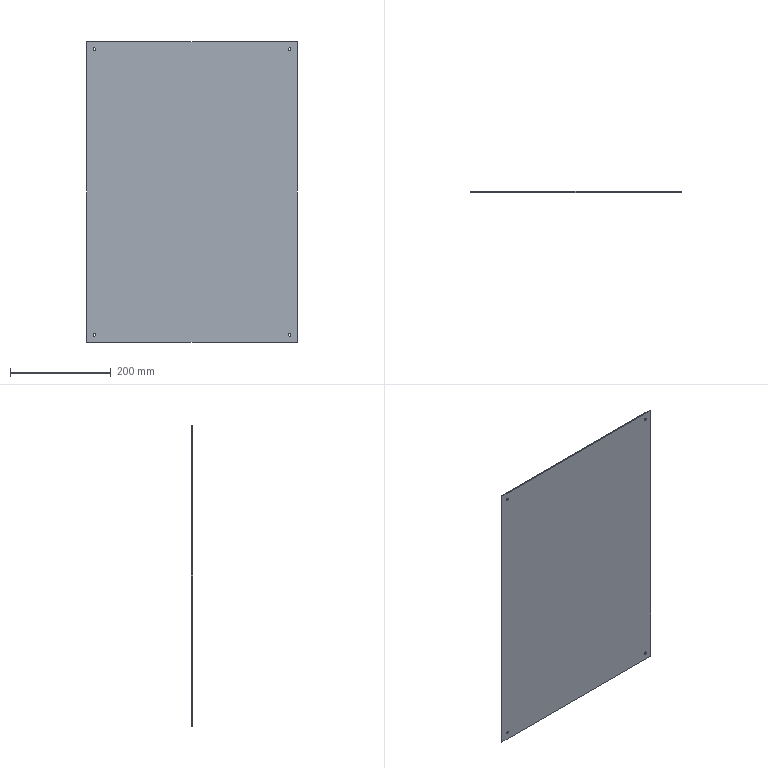Part | STEP file | PN_0007 (cover plate) | 1 solid | 14 faces | box 418 x 2 x 598 mm | volume 499771 mm3 | cylinder 8 | plane 6 | commonest cylinder face diameters 5 x8
STEP:
#1=CARTESIAN_POINT('',(0.,0.,0.));
#2=DIRECTION('',(0.,0.,1.));
#3=DIRECTION('',(1.,0.,0.));
#4=AXIS2_PLACEMENT_3D('',#1,#2,#3);
#5=CARTESIAN_POINT('',(-194.,-2.,286.5));
#6=VERTEX_POINT('',#5);
#7=CARTESIAN_POINT('',(-194.,0.,286.5));
#8=VERTEX_POINT('',#7);
#9=CARTESIAN_POINT('',(-194.,0.,286.5));
#10=DIRECTION('',(0.,1.,0.));
#11=VECTOR('',#10,1.);
#12=LINE('',#9,#11);
#13=CARTESIAN_POINT('',(-194.,0.,284.));
#14=DIRECTION('',(0.,1.,0.));
#15=DIRECTION('',(0.,0.,1.));
#16=AXIS2_PLACEMENT_3D('',#13,#14,#15);
#17=CYLINDRICAL_SURFACE('',#16,2.5);
#18=CARTESIAN_POINT('',(6.283,0.));
#19=DIRECTION('',(0.,1.));
#20=VECTOR('',#19,1.);
#21=LINE('',#18,#20);
#22=(GEOMETRIC_REPRESENTATION_CONTEXT(2)PARAMETRIC_REPRESENTATION_CONTEXT()REPRESENTATION_CONTEXT('',''));
#23=DEFINITIONAL_REPRESENTATION('',(#21),#22);
#24=PCURVE('',#17,#23);
#25=CARTESIAN_POINT('',(-194.,0.,284.));
#26=DIRECTION('',(0.,1.,0.));
#27=DIRECTION('',(0.,0.,1.));
#28=AXIS2_PLACEMENT_3D('',#25,#26,#27);
#29=CYLINDRICAL_SURFACE('',#28,2.5);
#30=CARTESIAN_POINT('',(0.,0.));
#31=DIRECTION('',(0.,1.));
#32=VECTOR('',#31,1.);
#33=LINE('',#30,#32);
#34=(GEOMETRIC_REPRESENTATION_CONTEXT(2)PARAMETRIC_REPRESENTATION_CONTEXT()REPRESENTATION_CONTEXT('',''));
#35=DEFINITIONAL_REPRESENTATION('',(#33),#34);
#36=PCURVE('',#29,#35);
#37=SURFACE_CURVE('',#12,(#24,#36),.PCURVE_S1.);
#38=EDGE_CURVE('',#6,#8,#37,.T.);
#39=ORIENTED_EDGE('',*,*,#38,.T.);
#40=CARTESIAN_POINT('',(-194.,0.,281.5));
#41=VERTEX_POINT('',#40);
#42=CARTESIAN_POINT('',(-194.,0.,284.));
#43=DIRECTION('',(0.,1.,0.));
#44=DIRECTION('',(0.,0.,1.));
#45=AXIS2_PLACEMENT_3D('',#42,#43,#44);
#46=CIRCLE('',#45,2.5);
#47=CARTESIAN_POINT('',(0.,0.));
#48=DIRECTION('',(1.,0.));
#49=VECTOR('',#48,1.);
#50=LINE('',#47,#49);
#51=(GEOMETRIC_REPRESENTATION_CONTEXT(2)PARAMETRIC_REPRESENTATION_CONTEXT()REPRESENTATION_CONTEXT('',''));
#52=DEFINITIONAL_REPRESENTATION('',(#50),#51);
#53=PCURVE('',#17,#52);
#54=CARTESIAN_POINT('',(0.,0.,0.));
#55=DIRECTION('',(0.,1.,0.));
#56=DIRECTION('',(0.,0.,1.));
#57=AXIS2_PLACEMENT_3D('',#54,#55,#56);
#58=PLANE('',#57);
#59=CARTESIAN_POINT('',(284.,-194.));
#60=DIRECTION('',(1.,0.));
#61=AXIS2_PLACEMENT_2D('',#59,#60);
#62=CIRCLE('',#61,2.5);
#63=(GEOMETRIC_REPRESENTATION_CONTEXT(2)PARAMETRIC_REPRESENTATION_CONTEXT()REPRESENTATION_CONTEXT('',''));
#64=DEFINITIONAL_REPRESENTATION('',(#62),#63);
#65=PCURVE('',#58,#64);
#66=SURFACE_CURVE('',#46,(#53,#65),.PCURVE_S1.);
#67=EDGE_CURVE('',#41,#8,#66,.T.);
#68=ORIENTED_EDGE('',*,*,#67,.F.);
#69=CARTESIAN_POINT('',(-194.,-2.,281.5));
#70=VERTEX_POINT('',#69);
#71=CARTESIAN_POINT('',(-194.,0.,281.5));
#72=DIRECTION('',(0.,1.,0.));
#73=VECTOR('',#72,1.);
#74=LINE('',#71,#73);
#75=CARTESIAN_POINT('',(3.142,0.));
#76=DIRECTION('',(0.,1.));
#77=VECTOR('',#76,1.);
#78=LINE('',#75,#77);
#79=(GEOMETRIC_REPRESENTATION_CONTEXT(2)PARAMETRIC_REPRESENTATION_CONTEXT()REPRESENTATION_CONTEXT('',''));
#80=DEFINITIONAL_REPRESENTATION('',(#78),#79);
#81=PCURVE('',#17,#80);
#82=CARTESIAN_POINT('',(3.142,0.));
#83=DIRECTION('',(0.,1.));
#84=VECTOR('',#83,1.);
#85=LINE('',#82,#84);
#86=(GEOMETRIC_REPRESENTATION_CONTEXT(2)PARAMETRIC_REPRESENTATION_CONTEXT()REPRESENTATION_CONTEXT('',''));
#87=DEFINITIONAL_REPRESENTATION('',(#85),#86);
#88=PCURVE('',#29,#87);
#89=SURFACE_CURVE('',#74,(#81,#88),.PCURVE_S1.);
#90=EDGE_CURVE('',#70,#41,#89,.T.);
#91=ORIENTED_EDGE('',*,*,#90,.F.);
#92=CARTESIAN_POINT('',(-194.,-2.,284.));
#93=DIRECTION('',(0.,1.,0.));
#94=DIRECTION('',(0.,0.,1.));
#95=AXIS2_PLACEMENT_3D('',#92,#93,#94);
#96=CIRCLE('',#95,2.5);
#97=CARTESIAN_POINT('',(0.,-2.));
#98=DIRECTION('',(1.,0.));
#99=VECTOR('',#98,1.);
#100=LINE('',#97,#99);
#101=(GEOMETRIC_REPRESENTATION_CONTEXT(2)PARAMETRIC_REPRESENTATION_CONTEXT()REPRESENTATION_CONTEXT('',''));
#102=DEFINITIONAL_REPRESENTATION('',(#100),#101);
#103=PCURVE('',#17,#102);
#104=CARTESIAN_POINT('',(0.,-2.,0.));
#105=DIRECTION('',(0.,1.,0.));
#106=DIRECTION('',(0.,0.,1.));
#107=AXIS2_PLACEMENT_3D('',#104,#105,#106);
#108=PLANE('',#107);
#109=CARTESIAN_POINT('',(284.,-194.));
#110=DIRECTION('',(1.,0.));
#111=AXIS2_PLACEMENT_2D('',#109,#110);
#112=CIRCLE('',#111,2.5);
#113=(GEOMETRIC_REPRESENTATION_CONTEXT(2)PARAMETRIC_REPRESENTATION_CONTEXT()REPRESENTATION_CONTEXT('',''));
#114=DEFINITIONAL_REPRESENTATION('',(#112),#113);
#115=PCURVE('',#108,#114);
#116=SURFACE_CURVE('',#96,(#103,#115),.PCURVE_S1.);
#117=EDGE_CURVE('',#70,#6,#116,.T.);
#118=ORIENTED_EDGE('',*,*,#117,.T.);
#119=EDGE_LOOP('',(#39,#68,#91,#118));
#120=FACE_BOUND('',#119,.F.);
#121=ADVANCED_FACE('',(#120),#17,.F.);
#122=CARTESIAN_POINT('',(194.,-2.,286.5));
#123=VERTEX_POINT('',#122);
#124=CARTESIAN_POINT('',(194.,0.,286.5));
#125=VERTEX_POINT('',#124);
#126=CARTESIAN_POINT('',(194.,0.,286.5));
#127=DIRECTION('',(0.,1.,0.));
#128=VECTOR('',#127,1.);
#129=LINE('',#126,#128);
#130=CARTESIAN_POINT('',(194.,0.,284.));
#131=DIRECTION('',(0.,1.,0.));
#132=DIRECTION('',(0.,0.,1.));
#133=AXIS2_PLACEMENT_3D('',#130,#131,#132);
#134=CYLINDRICAL_SURFACE('',#133,2.5);
#135=CARTESIAN_POINT('',(6.283,0.));
#136=DIRECTION('',(0.,1.));
#137=VECTOR('',#136,1.);
#138=LINE('',#135,#137);
#139=(GEOMETRIC_REPRESENTATION_CONTEXT(2)PARAMETRIC_REPRESENTATION_CONTEXT()REPRESENTATION_CONTEXT('',''));
#140=DEFINITIONAL_REPRESENTATION('',(#138),#139);
#141=PCURVE('',#134,#140);
#142=CARTESIAN_POINT('',(194.,0.,284.));
#143=DIRECTION('',(0.,1.,0.));
#144=DIRECTION('',(0.,0.,1.));
#145=AXIS2_PLACEMENT_3D('',#142,#143,#144);
#146=CYLINDRICAL_SURFACE('',#145,2.5);
#147=CARTESIAN_POINT('',(0.,0.));
#148=DIRECTION('',(0.,1.));
#149=VECTOR('',#148,1.);
#150=LINE('',#147,#149);
#151=(GEOMETRIC_REPRESENTATION_CONTEXT(2)PARAMETRIC_REPRESENTATION_CONTEXT()REPRESENTATION_CONTEXT('',''));
#152=DEFINITIONAL_REPRESENTATION('',(#150),#151);
#153=PCURVE('',#146,#152);
#154=SURFACE_CURVE('',#129,(#141,#153),.PCURVE_S1.);
#155=EDGE_CURVE('',#123,#125,#154,.T.);
#156=ORIENTED_EDGE('',*,*,#155,.T.);
#157=CARTESIAN_POINT('',(194.,0.,281.5));
#158=VERTEX_POINT('',#157);
#159=CARTESIAN_POINT('',(194.,0.,284.));
#160=DIRECTION('',(0.,1.,0.));
#161=DIRECTION('',(0.,0.,1.));
#162=AXIS2_PLACEMENT_3D('',#159,#160,#161);
#163=CIRCLE('',#162,2.5);
#164=CARTESIAN_POINT('',(0.,0.));
#165=DIRECTION('',(1.,0.));
#166=VECTOR('',#165,1.);
#167=LINE('',#164,#166);
#168=(GEOMETRIC_REPRESENTATION_CONTEXT(2)PARAMETRIC_REPRESENTATION_CONTEXT()REPRESENTATION_CONTEXT('',''));
#169=DEFINITIONAL_REPRESENTATION('',(#167),#168);
#170=PCURVE('',#134,#169);
#171=CARTESIAN_POINT('',(284.,194.));
#172=DIRECTION('',(1.,0.));
#173=AXIS2_PLACEMENT_2D('',#171,#172);
#174=CIRCLE('',#173,2.5);
#175=(GEOMETRIC_REPRESENTATION_CONTEXT(2)PARAMETRIC_REPRESENTATION_CONTEXT()REPRESENTATION_CONTEXT('',''));
#176=DEFINITIONAL_REPRESENTATION('',(#174),#175);
#177=PCURVE('',#58,#176);
#178=SURFACE_CURVE('',#163,(#170,#177),.PCURVE_S1.);
#179=EDGE_CURVE('',#158,#125,#178,.T.);
#180=ORIENTED_EDGE('',*,*,#179,.F.);
#181=CARTESIAN_POINT('',(194.,-2.,281.5));
#182=VERTEX_POINT('',#181);
#183=CARTESIAN_POINT('',(194.,0.,281.5));
#184=DIRECTION('',(0.,1.,0.));
#185=VECTOR('',#184,1.);
#186=LINE('',#183,#185);
#187=CARTESIAN_POINT('',(3.142,0.));
#188=DIRECTION('',(0.,1.));
#189=VECTOR('',#188,1.);
#190=LINE('',#187,#189);
#191=(GEOMETRIC_REPRESENTATION_CONTEXT(2)PARAMETRIC_REPRESENTATION_CONTEXT()REPRESENTATION_CONTEXT('',''));
#192=DEFINITIONAL_REPRESENTATION('',(#190),#191);
#193=PCURVE('',#134,#192);
#194=CARTESIAN_POINT('',(3.142,0.));
#195=DIRECTION('',(0.,1.));
#196=VECTOR('',#195,1.);
#197=LINE('',#194,#196);
#198=(GEOMETRIC_REPRESENTATION_CONTEXT(2)PARAMETRIC_REPRESENTATION_CONTEXT()REPRESENTATION_CONTEXT('',''));
#199=DEFINITIONAL_REPRESENTATION('',(#197),#198);
#200=PCURVE('',#146,#199);
#201=SURFACE_CURVE('',#186,(#193,#200),.PCURVE_S1.);
#202=EDGE_CURVE('',#182,#158,#201,.T.);
#203=ORIENTED_EDGE('',*,*,#202,.F.);
#204=CARTESIAN_POINT('',(194.,-2.,284.));
#205=DIRECTION('',(0.,1.,0.));
#206=DIRECTION('',(0.,0.,1.));
#207=AXIS2_PLACEMENT_3D('',#204,#205,#206);
#208=CIRCLE('',#207,2.5);
#209=CARTESIAN_POINT('',(0.,-2.));
#210=DIRECTION('',(1.,0.));
#211=VECTOR('',#210,1.);
#212=LINE('',#209,#211);
#213=(GEOMETRIC_REPRESENTATION_CONTEXT(2)PARAMETRIC_REPRESENTATION_CONTEXT()REPRESENTATION_CONTEXT('',''));
#214=DEFINITIONAL_REPRESENTATION('',(#212),#213);
#215=PCURVE('',#134,#214);
#216=CARTESIAN_POINT('',(284.,194.));
#217=DIRECTION('',(1.,0.));
#218=AXIS2_PLACEMENT_2D('',#216,#217);
#219=CIRCLE('',#218,2.5);
#220=(GEOMETRIC_REPRESENTATION_CONTEXT(2)PARAMETRIC_REPRESENTATION_CONTEXT()REPRESENTATION_CONTEXT('',''));
#221=DEFINITIONAL_REPRESENTATION('',(#219),#220);
#222=PCURVE('',#108,#221);
#223=SURFACE_CURVE('',#208,(#215,#222),.PCURVE_S1.);
#224=EDGE_CURVE('',#182,#123,#223,.T.);
#225=ORIENTED_EDGE('',*,*,#224,.T.);
#226=EDGE_LOOP('',(#156,#180,#203,#225));
#227=FACE_BOUND('',#226,.F.);
#228=ADVANCED_FACE('',(#227),#134,.F.);
#229=CARTESIAN_POINT('',(194.,-2.,-281.5));
#230=VERTEX_POINT('',#229);
#231=CARTESIAN_POINT('',(194.,0.,-281.5));
#232=VERTEX_POINT('',#231);
#233=CARTESIAN_POINT('',(194.,0.,-281.5));
#234=DIRECTION('',(0.,1.,0.));
#235=VECTOR('',#234,1.);
#236=LINE('',#233,#235);
#237=CARTESIAN_POINT('',(194.,0.,-284.));
#238=DIRECTION('',(0.,1.,0.));
#239=DIRECTION('',(0.,0.,1.));
#240=AXIS2_PLACEMENT_3D('',#237,#238,#239);
#241=CYLINDRICAL_SURFACE('',#240,2.5);
#242=CARTESIAN_POINT('',(6.283,0.));
#243=DIRECTION('',(0.,1.));
#244=VECTOR('',#243,1.);
#245=LINE('',#242,#244);
#246=(GEOMETRIC_REPRESENTATION_CONTEXT(2)PARAMETRIC_REPRESENTATION_CONTEXT()REPRESENTATION_CONTEXT('',''));
#247=DEFINITIONAL_REPRESENTATION('',(#245),#246);
#248=PCURVE('',#241,#247);
#249=CARTESIAN_POINT('',(194.,0.,-284.));
#250=DIRECTION('',(0.,1.,0.));
#251=DIRECTION('',(0.,0.,1.));
#252=AXIS2_PLACEMENT_3D('',#249,#250,#251);
#253=CYLINDRICAL_SURFACE('',#252,2.5);
#254=CARTESIAN_POINT('',(0.,0.));
#255=DIRECTION('',(0.,1.));
#256=VECTOR('',#255,1.);
#257=LINE('',#254,#256);
#258=(GEOMETRIC_REPRESENTATION_CONTEXT(2)PARAMETRIC_REPRESENTATION_CONTEXT()REPRESENTATION_CONTEXT('',''));
#259=DEFINITIONAL_REPRESENTATION('',(#257),#258);
#260=PCURVE('',#253,#259);
#261=SURFACE_CURVE('',#236,(#248,#260),.PCURVE_S1.);
#262=EDGE_CURVE('',#230,#232,#261,.T.);
#263=ORIENTED_EDGE('',*,*,#262,.T.);
#264=CARTESIAN_POINT('',(194.,0.,-286.5));
#265=VERTEX_POINT('',#264);
#266=CARTESIAN_POINT('',(194.,0.,-284.));
#267=DIRECTION('',(0.,1.,0.));
#268=DIRECTION('',(0.,0.,1.));
#269=AXIS2_PLACEMENT_3D('',#266,#267,#268);
#270=CIRCLE('',#269,2.5);
#271=CARTESIAN_POINT('',(0.,0.));
#272=DIRECTION('',(1.,0.));
#273=VECTOR('',#272,1.);
#274=LINE('',#271,#273);
#275=(GEOMETRIC_REPRESENTATION_CONTEXT(2)PARAMETRIC_REPRESENTATION_CONTEXT()REPRESENTATION_CONTEXT('',''));
#276=DEFINITIONAL_REPRESENTATION('',(#274),#275);
#277=PCURVE('',#241,#276);
#278=CARTESIAN_POINT('',(-284.,194.));
#279=DIRECTION('',(1.,0.));
#280=AXIS2_PLACEMENT_2D('',#278,#279);
#281=CIRCLE('',#280,2.5);
#282=(GEOMETRIC_REPRESENTATION_CONTEXT(2)PARAMETRIC_REPRESENTATION_CONTEXT()REPRESENTATION_CONTEXT('',''));
#283=DEFINITIONAL_REPRESENTATION('',(#281),#282);
#284=PCURVE('',#58,#283);
#285=SURFACE_CURVE('',#270,(#277,#284),.PCURVE_S1.);
#286=EDGE_CURVE('',#265,#232,#285,.T.);
#287=ORIENTED_EDGE('',*,*,#286,.F.);
#288=CARTESIAN_POINT('',(194.,-2.,-286.5));
#289=VERTEX_POINT('',#288);
#290=CARTESIAN_POINT('',(194.,0.,-286.5));
#291=DIRECTION('',(0.,1.,0.));
#292=VECTOR('',#291,1.);
#293=LINE('',#290,#292);
#294=CARTESIAN_POINT('',(3.142,0.));
#295=DIRECTION('',(0.,1.));
#296=VECTOR('',#295,1.);
#297=LINE('',#294,#296);
#298=(GEOMETRIC_REPRESENTATION_CONTEXT(2)PARAMETRIC_REPRESENTATION_CONTEXT()REPRESENTATION_CONTEXT('',''));
#299=DEFINITIONAL_REPRESENTATION('',(#297),#298);
#300=PCURVE('',#241,#299);
#301=CARTESIAN_POINT('',(3.142,0.));
#302=DIRECTION('',(0.,1.));
#303=VECTOR('',#302,1.);
#304=LINE('',#301,#303);
#305=(GEOMETRIC_REPRESENTATION_CONTEXT(2)PARAMETRIC_REPRESENTATION_CONTEXT()REPRESENTATION_CONTEXT('',''));
#306=DEFINITIONAL_REPRESENTATION('',(#304),#305);
#307=PCURVE('',#253,#306);
#308=SURFACE_CURVE('',#293,(#300,#307),.PCURVE_S1.);
#309=EDGE_CURVE('',#289,#265,#308,.T.);
#310=ORIENTED_EDGE('',*,*,#309,.F.);
#311=CARTESIAN_POINT('',(194.,-2.,-284.));
#312=DIRECTION('',(0.,1.,0.));
#313=DIRECTION('',(0.,0.,1.));
#314=AXIS2_PLACEMENT_3D('',#311,#312,#313);
#315=CIRCLE('',#314,2.5);
#316=CARTESIAN_POINT('',(0.,-2.));
#317=DIRECTION('',(1.,0.));
#318=VECTOR('',#317,1.);
#319=LINE('',#316,#318);
#320=(GEOMETRIC_REPRESENTATION_CONTEXT(2)PARAMETRIC_REPRESENTATION_CONTEXT()REPRESENTATION_CONTEXT('',''));
#321=DEFINITIONAL_REPRESENTATION('',(#319),#320);
#322=PCURVE('',#241,#321);
#323=CARTESIAN_POINT('',(-284.,194.));
#324=DIRECTION('',(1.,0.));
#325=AXIS2_PLACEMENT_2D('',#323,#324);
#326=CIRCLE('',#325,2.5);
#327=(GEOMETRIC_REPRESENTATION_CONTEXT(2)PARAMETRIC_REPRESENTATION_CONTEXT()REPRESENTATION_CONTEXT('',''));
#328=DEFINITIONAL_REPRESENTATION('',(#326),#327);
#329=PCURVE('',#108,#328);
#330=SURFACE_CURVE('',#315,(#322,#329),.PCURVE_S1.);
#331=EDGE_CURVE('',#289,#230,#330,.T.);
#332=ORIENTED_EDGE('',*,*,#331,.T.);
#333=EDGE_LOOP('',(#263,#287,#310,#332));
#334=FACE_BOUND('',#333,.F.);
#335=ADVANCED_FACE('',(#334),#241,.F.);
#336=CARTESIAN_POINT('',(-194.,-2.,-281.5));
#337=VERTEX_POINT('',#336);
#338=CARTESIAN_POINT('',(-194.,0.,-281.5));
#339=VERTEX_POINT('',#338);
#340=CARTESIAN_POINT('',(-194.,0.,-281.5));
#341=DIRECTION('',(0.,1.,0.));
#342=VECTOR('',#341,1.);
#343=LINE('',#340,#342);
#344=CARTESIAN_POINT('',(-194.,0.,-284.));
#345=DIRECTION('',(0.,1.,0.));
#346=DIRECTION('',(0.,0.,1.));
#347=AXIS2_PLACEMENT_3D('',#344,#345,#346);
#348=CYLINDRICAL_SURFACE('',#347,2.5);
#349=CARTESIAN_POINT('',(6.283,0.));
#350=DIRECTION('',(0.,1.));
#351=VECTOR('',#350,1.);
#352=LINE('',#349,#351);
#353=(GEOMETRIC_REPRESENTATION_CONTEXT(2)PARAMETRIC_REPRESENTATION_CONTEXT()REPRESENTATION_CONTEXT('',''));
#354=DEFINITIONAL_REPRESENTATION('',(#352),#353);
#355=PCURVE('',#348,#354);
#356=CARTESIAN_POINT('',(-194.,0.,-284.));
#357=DIRECTION('',(0.,1.,0.));
#358=DIRECTION('',(0.,0.,1.));
#359=AXIS2_PLACEMENT_3D('',#356,#357,#358);
#360=CYLINDRICAL_SURFACE('',#359,2.5);
#361=CARTESIAN_POINT('',(0.,0.));
#362=DIRECTION('',(0.,1.));
#363=VECTOR('',#362,1.);
#364=LINE('',#361,#363);
#365=(GEOMETRIC_REPRESENTATION_CONTEXT(2)PARAMETRIC_REPRESENTATION_CONTEXT()REPRESENTATION_CONTEXT('',''));
#366=DEFINITIONAL_REPRESENTATION('',(#364),#365);
#367=PCURVE('',#360,#366);
#368=SURFACE_CURVE('',#343,(#355,#367),.PCURVE_S1.);
#369=EDGE_CURVE('',#337,#339,#368,.T.);
#370=ORIENTED_EDGE('',*,*,#369,.T.);
#371=CARTESIAN_POINT('',(-194.,0.,-286.5));
#372=VERTEX_POINT('',#371);
#373=CARTESIAN_POINT('',(-194.,0.,-284.));
#374=DIRECTION('',(0.,1.,0.));
#375=DIRECTION('',(0.,0.,1.));
#376=AXIS2_PLACEMENT_3D('',#373,#374,#375);
#377=CIRCLE('',#376,2.5);
#378=CARTESIAN_POINT('',(0.,0.));
#379=DIRECTION('',(1.,0.));
#380=VECTOR('',#379,1.);
#381=LINE('',#378,#380);
#382=(GEOMETRIC_REPRESENTATION_CONTEXT(2)PARAMETRIC_REPRESENTATION_CONTEXT()REPRESENTATION_CONTEXT('',''));
#383=DEFINITIONAL_REPRESENTATION('',(#381),#382);
#384=PCURVE('',#348,#383);
#385=CARTESIAN_POINT('',(-284.,-194.));
#386=DIRECTION('',(1.,0.));
#387=AXIS2_PLACEMENT_2D('',#385,#386);
#388=CIRCLE('',#387,2.5);
#389=(GEOMETRIC_REPRESENTATION_CONTEXT(2)PARAMETRIC_REPRESENTATION_CONTEXT()REPRESENTATION_CONTEXT('',''));
#390=DEFINITIONAL_REPRESENTATION('',(#388),#389);
#391=PCURVE('',#58,#390);
#392=SURFACE_CURVE('',#377,(#384,#391),.PCURVE_S1.);
#393=EDGE_CURVE('',#372,#339,#392,.T.);
#394=ORIENTED_EDGE('',*,*,#393,.F.);
#395=CARTESIAN_POINT('',(-194.,-2.,-286.5));
#396=VERTEX_POINT('',#395);
#397=CARTESIAN_POINT('',(-194.,0.,-286.5));
#398=DIRECTION('',(0.,1.,0.));
#399=VECTOR('',#398,1.);
#400=LINE('',#397,#399);
#401=CARTESIAN_POINT('',(3.142,0.));
#402=DIRECTION('',(0.,1.));
#403=VECTOR('',#402,1.);
#404=LINE('',#401,#403);
#405=(GEOMETRIC_REPRESENTATION_CONTEXT(2)PARAMETRIC_REPRESENTATION_CONTEXT()REPRESENTATION_CONTEXT('',''));
#406=DEFINITIONAL_REPRESENTATION('',(#404),#405);
#407=PCURVE('',#348,#406);
#408=CARTESIAN_POINT('',(3.142,0.));
#409=DIRECTION('',(0.,1.));
#410=VECTOR('',#409,1.);
#411=LINE('',#408,#410);
#412=(GEOMETRIC_REPRESENTATION_CONTEXT(2)PARAMETRIC_REPRESENTATION_CONTEXT()REPRESENTATION_CONTEXT('',''));
#413=DEFINITIONAL_REPRESENTATION('',(#411),#412);
#414=PCURVE('',#360,#413);
#415=SURFACE_CURVE('',#400,(#407,#414),.PCURVE_S1.);
#416=EDGE_CURVE('',#396,#372,#415,.T.);
#417=ORIENTED_EDGE('',*,*,#416,.F.);
#418=CARTESIAN_POINT('',(-194.,-2.,-284.));
#419=DIRECTION('',(0.,1.,0.));
#420=DIRECTION('',(0.,0.,1.));
#421=AXIS2_PLACEMENT_3D('',#418,#419,#420);
#422=CIRCLE('',#421,2.5);
#423=CARTESIAN_POINT('',(0.,-2.));
#424=DIRECTION('',(1.,0.));
#425=VECTOR('',#424,1.);
#426=LINE('',#423,#425);
#427=(GEOMETRIC_REPRESENTATION_CONTEXT(2)PARAMETRIC_REPRESENTATION_CONTEXT()REPRESENTATION_CONTEXT('',''));
#428=DEFINITIONAL_REPRESENTATION('',(#426),#427);
#429=PCURVE('',#348,#428);
#430=CARTESIAN_POINT('',(-284.,-194.));
#431=DIRECTION('',(1.,0.));
#432=AXIS2_PLACEMENT_2D('',#430,#431);
#433=CIRCLE('',#432,2.5);
#434=(GEOMETRIC_REPRESENTATION_CONTEXT(2)PARAMETRIC_REPRESENTATION_CONTEXT()REPRESENTATION_CONTEXT('',''));
#435=DEFINITIONAL_REPRESENTATION('',(#433),#434);
#436=PCURVE('',#108,#435);
#437=SURFACE_CURVE('',#422,(#429,#436),.PCURVE_S1.);
#438=EDGE_CURVE('',#396,#337,#437,.T.);
#439=ORIENTED_EDGE('',*,*,#438,.T.);
#440=EDGE_LOOP('',(#370,#394,#417,#439));
#441=FACE_BOUND('',#440,.F.);
#442=ADVANCED_FACE('',(#441),#348,.F.);
#443=CARTESIAN_POINT('',(-209.,0.,299.));
#444=VERTEX_POINT('',#443);
#445=CARTESIAN_POINT('',(209.,0.,299.));
#446=VERTEX_POINT('',#445);
#447=CARTESIAN_POINT('',(209.,0.,299.));
#448=DIRECTION('',(1.,0.,0.));
#449=VECTOR('',#448,1.);
#450=LINE('',#447,#449);
#451=CARTESIAN_POINT('',(209.,-2.,299.));
#452=DIRECTION('',(0.,0.,1.));
#453=DIRECTION('',(1.,0.,0.));
#454=AXIS2_PLACEMENT_3D('',#451,#452,#453);
#455=PLANE('',#454);
#456=CARTESIAN_POINT('',(0.,2.));
#457=DIRECTION('',(1.,0.));
#458=VECTOR('',#457,1.);
#459=LINE('',#456,#458);
#460=(GEOMETRIC_REPRESENTATION_CONTEXT(2)PARAMETRIC_REPRESENTATION_CONTEXT()REPRESENTATION_CONTEXT('',''));
#461=DEFINITIONAL_REPRESENTATION('',(#459),#460);
#462=PCURVE('',#455,#461);
#463=CARTESIAN_POINT('',(299.,209.));
#464=DIRECTION('',(0.,1.));
#465=VECTOR('',#464,1.);
#466=LINE('',#463,#465);
#467=(GEOMETRIC_REPRESENTATION_CONTEXT(2)PARAMETRIC_REPRESENTATION_CONTEXT()REPRESENTATION_CONTEXT('',''));
#468=DEFINITIONAL_REPRESENTATION('',(#466),#467);
#469=PCURVE('',#58,#468);
#470=SURFACE_CURVE('',#450,(#462,#469),.PCURVE_S1.);
#471=EDGE_CURVE('',#444,#446,#470,.T.);
#472=ORIENTED_EDGE('',*,*,#471,.F.);
#473=CARTESIAN_POINT('',(-209.,-2.,299.));
#474=VERTEX_POINT('',#473);
#475=CARTESIAN_POINT('',(-209.,-2.,299.));
#476=DIRECTION('',(0.,1.,0.));
#477=VECTOR('',#476,1.);
#478=LINE('',#475,#477);
#479=CARTESIAN_POINT('',(-418.,0.));
#480=DIRECTION('',(0.,1.));
#481=VECTOR('',#480,1.);
#482=LINE('',#479,#481);
#483=(GEOMETRIC_REPRESENTATION_CONTEXT(2)PARAMETRIC_REPRESENTATION_CONTEXT()REPRESENTATION_CONTEXT('',''));
#484=DEFINITIONAL_REPRESENTATION('',(#482),#483);
#485=PCURVE('',#455,#484);
#486=CARTESIAN_POINT('',(-209.,-2.,-299.));
#487=DIRECTION('',(-1.,0.,0.));
#488=DIRECTION('',(0.,0.,1.));
#489=AXIS2_PLACEMENT_3D('',#486,#487,#488);
#490=PLANE('',#489);
#491=CARTESIAN_POINT('',(598.,0.));
#492=DIRECTION('',(0.,1.));
#493=VECTOR('',#492,1.);
#494=LINE('',#491,#493);
#495=(GEOMETRIC_REPRESENTATION_CONTEXT(2)PARAMETRIC_REPRESENTATION_CONTEXT()REPRESENTATION_CONTEXT('',''));
#496=DEFINITIONAL_REPRESENTATION('',(#494),#495);
#497=PCURVE('',#490,#496);
#498=SURFACE_CURVE('',#478,(#485,#497),.PCURVE_S1.);
#499=EDGE_CURVE('',#474,#444,#498,.T.);
#500=ORIENTED_EDGE('',*,*,#499,.F.);
#501=CARTESIAN_POINT('',(209.,-2.,299.));
#502=VERTEX_POINT('',#501);
#503=CARTESIAN_POINT('',(209.,-2.,299.));
#504=DIRECTION('',(1.,0.,0.));
#505=VECTOR('',#504,1.);
#506=LINE('',#503,#505);
#507=CARTESIAN_POINT('',(0.,0.));
#508=DIRECTION('',(1.,0.));
#509=VECTOR('',#508,1.);
#510=LINE('',#507,#509);
#511=(GEOMETRIC_REPRESENTATION_CONTEXT(2)PARAMETRIC_REPRESENTATION_CONTEXT()REPRESENTATION_CONTEXT('',''));
#512=DEFINITIONAL_REPRESENTATION('',(#510),#511);
#513=PCURVE('',#455,#512);
#514=CARTESIAN_POINT('',(299.,209.));
#515=DIRECTION('',(0.,1.));
#516=VECTOR('',#515,1.);
#517=LINE('',#514,#516);
#518=(GEOMETRIC_REPRESENTATION_CONTEXT(2)PARAMETRIC_REPRESENTATION_CONTEXT()REPRESENTATION_CONTEXT('',''));
#519=DEFINITIONAL_REPRESENTATION('',(#517),#518);
#520=PCURVE('',#108,#519);
#521=SURFACE_CURVE('',#506,(#513,#520),.PCURVE_S1.);
#522=EDGE_CURVE('',#474,#502,#521,.T.);
#523=ORIENTED_EDGE('',*,*,#522,.T.);
#524=CARTESIAN_POINT('',(209.,-2.,299.));
#525=DIRECTION('',(0.,1.,0.));
#526=VECTOR('',#525,1.);
#527=LINE('',#524,#526);
#528=CARTESIAN_POINT('',(0.,0.));
#529=DIRECTION('',(0.,1.));
#530=VECTOR('',#529,1.);
#531=LINE('',#528,#530);
#532=(GEOMETRIC_REPRESENTATION_CONTEXT(2)PARAMETRIC_REPRESENTATION_CONTEXT()REPRESENTATION_CONTEXT('',''));
#533=DEFINITIONAL_REPRESENTATION('',(#531),#532);
#534=PCURVE('',#455,#533);
#535=CARTESIAN_POINT('',(209.,-2.,-299.));
#536=DIRECTION('',(1.,0.,0.));
#537=DIRECTION('',(0.,0.,-1.));
#538=AXIS2_PLACEMENT_3D('',#535,#536,#537);
#539=PLANE('',#538);
#540=CARTESIAN_POINT('',(-598.,0.));
#541=DIRECTION('',(0.,1.));
#542=VECTOR('',#541,1.);
#543=LINE('',#540,#542);
#544=(GEOMETRIC_REPRESENTATION_CONTEXT(2)PARAMETRIC_REPRESENTATION_CONTEXT()REPRESENTATION_CONTEXT('',''));
#545=DEFINITIONAL_REPRESENTATION('',(#543),#544);
#546=PCURVE('',#539,#545);
#547=SURFACE_CURVE('',#527,(#534,#546),.PCURVE_S1.);
#548=EDGE_CURVE('',#502,#446,#547,.T.);
#549=ORIENTED_EDGE('',*,*,#548,.T.);
#550=EDGE_LOOP('',(#472,#500,#523,#549));
#551=FACE_BOUND('',#550,.T.);
#552=ADVANCED_FACE('',(#551),#455,.T.);
#553=CARTESIAN_POINT('',(-209.,0.,-299.));
#554=VERTEX_POINT('',#553);
#555=CARTESIAN_POINT('',(-209.,0.,-299.));
#556=DIRECTION('',(0.,0.,1.));
#557=VECTOR('',#556,1.);
#558=LINE('',#555,#557);
#559=CARTESIAN_POINT('',(0.,2.));
#560=DIRECTION('',(1.,0.));
#561=VECTOR('',#560,1.);
#562=LINE('',#559,#561);
#563=(GEOMETRIC_REPRESENTATION_CONTEXT(2)PARAMETRIC_REPRESENTATION_CONTEXT()REPRESENTATION_CONTEXT('',''));
#564=DEFINITIONAL_REPRESENTATION('',(#562),#563);
#565=PCURVE('',#490,#564);
#566=CARTESIAN_POINT('',(-299.,-209.));
#567=DIRECTION('',(1.,0.));
#568=VECTOR('',#567,1.);
#569=LINE('',#566,#568);
#570=(GEOMETRIC_REPRESENTATION_CONTEXT(2)PARAMETRIC_REPRESENTATION_CONTEXT()REPRESENTATION_CONTEXT('',''));
#571=DEFINITIONAL_REPRESENTATION('',(#569),#570);
#572=PCURVE('',#58,#571);
#573=SURFACE_CURVE('',#558,(#565,#572),.PCURVE_S1.);
#574=EDGE_CURVE('',#554,#444,#573,.T.);
#575=ORIENTED_EDGE('',*,*,#574,.F.);
#576=CARTESIAN_POINT('',(-209.,-2.,-299.));
#577=VERTEX_POINT('',#576);
#578=CARTESIAN_POINT('',(-209.,-2.,-299.));
#579=DIRECTION('',(0.,1.,0.));
#580=VECTOR('',#579,1.);
#581=LINE('',#578,#580);
#582=CARTESIAN_POINT('',(0.,0.));
#583=DIRECTION('',(0.,1.));
#584=VECTOR('',#583,1.);
#585=LINE('',#582,#584);
#586=(GEOMETRIC_REPRESENTATION_CONTEXT(2)PARAMETRIC_REPRESENTATION_CONTEXT()REPRESENTATION_CONTEXT('',''));
#587=DEFINITIONAL_REPRESENTATION('',(#585),#586);
#588=PCURVE('',#490,#587);
#589=CARTESIAN_POINT('',(209.,-2.,-299.));
#590=DIRECTION('',(0.,0.,-1.));
#591=DIRECTION('',(-1.,0.,0.));
#592=AXIS2_PLACEMENT_3D('',#589,#590,#591);
#593=PLANE('',#592);
#594=CARTESIAN_POINT('',(418.,0.));
#595=DIRECTION('',(0.,1.));
#596=VECTOR('',#595,1.);
#597=LINE('',#594,#596);
#598=(GEOMETRIC_REPRESENTATION_CONTEXT(2)PARAMETRIC_REPRESENTATION_CONTEXT()REPRESENTATION_CONTEXT('',''));
#599=DEFINITIONAL_REPRESENTATION('',(#597),#598);
#600=PCURVE('',#593,#599);
#601=SURFACE_CURVE('',#581,(#588,#600),.PCURVE_S1.);
#602=EDGE_CURVE('',#577,#554,#601,.T.);
#603=ORIENTED_EDGE('',*,*,#602,.F.);
#604=CARTESIAN_POINT('',(-209.,-2.,-299.));
#605=DIRECTION('',(0.,0.,1.));
#606=VECTOR('',#605,1.);
#607=LINE('',#604,#606);
#608=CARTESIAN_POINT('',(0.,0.));
#609=DIRECTION('',(1.,0.));
#610=VECTOR('',#609,1.);
#611=LINE('',#608,#610);
#612=(GEOMETRIC_REPRESENTATION_CONTEXT(2)PARAMETRIC_REPRESENTATION_CONTEXT()REPRESENTATION_CONTEXT('',''));
#613=DEFINITIONAL_REPRESENTATION('',(#611),#612);
#614=PCURVE('',#490,#613);
#615=CARTESIAN_POINT('',(-299.,-209.));
#616=DIRECTION('',(1.,0.));
#617=VECTOR('',#616,1.);
#618=LINE('',#615,#617);
#619=(GEOMETRIC_REPRESENTATION_CONTEXT(2)PARAMETRIC_REPRESENTATION_CONTEXT()REPRESENTATION_CONTEXT('',''));
#620=DEFINITIONAL_REPRESENTATION('',(#618),#619);
#621=PCURVE('',#108,#620);
#622=SURFACE_CURVE('',#607,(#614,#621),.PCURVE_S1.);
#623=EDGE_CURVE('',#577,#474,#622,.T.);
#624=ORIENTED_EDGE('',*,*,#623,.T.);
#625=ORIENTED_EDGE('',*,*,#499,.T.);
#626=EDGE_LOOP('',(#575,#603,#624,#625));
#627=FACE_BOUND('',#626,.T.);
#628=ADVANCED_FACE('',(#627),#490,.T.);
#629=CARTESIAN_POINT('',(209.,0.,-299.));
#630=VERTEX_POINT('',#629);
#631=CARTESIAN_POINT('',(209.,0.,-299.));
#632=DIRECTION('',(-1.,0.,0.));
#633=VECTOR('',#632,1.);
#634=LINE('',#631,#633);
#635=CARTESIAN_POINT('',(0.,2.));
#636=DIRECTION('',(1.,0.));
#637=VECTOR('',#636,1.);
#638=LINE('',#635,#637);
#639=(GEOMETRIC_REPRESENTATION_CONTEXT(2)PARAMETRIC_REPRESENTATION_CONTEXT()REPRESENTATION_CONTEXT('',''));
#640=DEFINITIONAL_REPRESENTATION('',(#638),#639);
#641=PCURVE('',#593,#640);
#642=CARTESIAN_POINT('',(-299.,209.));
#643=DIRECTION('',(0.,-1.));
#644=VECTOR('',#643,1.);
#645=LINE('',#642,#644);
#646=(GEOMETRIC_REPRESENTATION_CONTEXT(2)PARAMETRIC_REPRESENTATION_CONTEXT()REPRESENTATION_CONTEXT('',''));
#647=DEFINITIONAL_REPRESENTATION('',(#645),#646);
#648=PCURVE('',#58,#647);
#649=SURFACE_CURVE('',#634,(#641,#648),.PCURVE_S1.);
#650=EDGE_CURVE('',#630,#554,#649,.T.);
#651=ORIENTED_EDGE('',*,*,#650,.F.);
#652=CARTESIAN_POINT('',(209.,-2.,-299.));
#653=VERTEX_POINT('',#652);
#654=CARTESIAN_POINT('',(209.,-2.,-299.));
#655=DIRECTION('',(0.,1.,0.));
#656=VECTOR('',#655,1.);
#657=LINE('',#654,#656);
#658=CARTESIAN_POINT('',(0.,0.));
#659=DIRECTION('',(0.,1.));
#660=VECTOR('',#659,1.);
#661=LINE('',#658,#660);
#662=(GEOMETRIC_REPRESENTATION_CONTEXT(2)PARAMETRIC_REPRESENTATION_CONTEXT()REPRESENTATION_CONTEXT('',''));
#663=DEFINITIONAL_REPRESENTATION('',(#661),#662);
#664=PCURVE('',#593,#663);
#665=CARTESIAN_POINT('',(0.,0.));
#666=DIRECTION('',(0.,1.));
#667=VECTOR('',#666,1.);
#668=LINE('',#665,#667);
#669=(GEOMETRIC_REPRESENTATION_CONTEXT(2)PARAMETRIC_REPRESENTATION_CONTEXT()REPRESENTATION_CONTEXT('',''));
#670=DEFINITIONAL_REPRESENTATION('',(#668),#669);
#671=PCURVE('',#539,#670);
#672=SURFACE_CURVE('',#657,(#664,#671),.PCURVE_S1.);
#673=EDGE_CURVE('',#653,#630,#672,.T.);
#674=ORIENTED_EDGE('',*,*,#673,.F.);
#675=CARTESIAN_POINT('',(209.,-2.,-299.));
#676=DIRECTION('',(-1.,0.,0.));
#677=VECTOR('',#676,1.);
#678=LINE('',#675,#677);
#679=CARTESIAN_POINT('',(0.,0.));
#680=DIRECTION('',(1.,0.));
#681=VECTOR('',#680,1.);
#682=LINE('',#679,#681);
#683=(GEOMETRIC_REPRESENTATION_CONTEXT(2)PARAMETRIC_REPRESENTATION_CONTEXT()REPRESENTATION_CONTEXT('',''));
#684=DEFINITIONAL_REPRESENTATION('',(#682),#683);
#685=PCURVE('',#593,#684);
#686=CARTESIAN_POINT('',(-299.,209.));
#687=DIRECTION('',(0.,-1.));
#688=VECTOR('',#687,1.);
#689=LINE('',#686,#688);
#690=(GEOMETRIC_REPRESENTATION_CONTEXT(2)PARAMETRIC_REPRESENTATION_CONTEXT()REPRESENTATION_CONTEXT('',''));
#691=DEFINITIONAL_REPRESENTATION('',(#689),#690);
#692=PCURVE('',#108,#691);
#693=SURFACE_CURVE('',#678,(#685,#692),.PCURVE_S1.);
#694=EDGE_CURVE('',#653,#577,#693,.T.);
#695=ORIENTED_EDGE('',*,*,#694,.T.);
#696=ORIENTED_EDGE('',*,*,#602,.T.);
#697=EDGE_LOOP('',(#651,#674,#695,#696));
#698=FACE_BOUND('',#697,.T.);
#699=ADVANCED_FACE('',(#698),#593,.T.);
#700=CARTESIAN_POINT('',(209.,0.,-299.));
#701=DIRECTION('',(0.,0.,-1.));
#702=VECTOR('',#701,1.);
#703=LINE('',#700,#702);
#704=CARTESIAN_POINT('',(0.,2.));
#705=DIRECTION('',(1.,0.));
#706=VECTOR('',#705,1.);
#707=LINE('',#704,#706);
#708=(GEOMETRIC_REPRESENTATION_CONTEXT(2)PARAMETRIC_REPRESENTATION_CONTEXT()REPRESENTATION_CONTEXT('',''));
#709=DEFINITIONAL_REPRESENTATION('',(#707),#708);
#710=PCURVE('',#539,#709);
#711=CARTESIAN_POINT('',(-299.,209.));
#712=DIRECTION('',(-1.,0.));
#713=VECTOR('',#712,1.);
#714=LINE('',#711,#713);
#715=(GEOMETRIC_REPRESENTATION_CONTEXT(2)PARAMETRIC_REPRESENTATION_CONTEXT()REPRESENTATION_CONTEXT('',''));
#716=DEFINITIONAL_REPRESENTATION('',(#714),#715);
#717=PCURVE('',#58,#716);
#718=SURFACE_CURVE('',#703,(#710,#717),.PCURVE_S1.);
#719=EDGE_CURVE('',#446,#630,#718,.T.);
#720=ORIENTED_EDGE('',*,*,#719,.F.);
#721=ORIENTED_EDGE('',*,*,#548,.F.);
#722=CARTESIAN_POINT('',(209.,-2.,-299.));
#723=DIRECTION('',(0.,0.,-1.));
#724=VECTOR('',#723,1.);
#725=LINE('',#722,#724);
#726=CARTESIAN_POINT('',(0.,0.));
#727=DIRECTION('',(1.,0.));
#728=VECTOR('',#727,1.);
#729=LINE('',#726,#728);
#730=(GEOMETRIC_REPRESENTATION_CONTEXT(2)PARAMETRIC_REPRESENTATION_CONTEXT()REPRESENTATION_CONTEXT('',''));
#731=DEFINITIONAL_REPRESENTATION('',(#729),#730);
#732=PCURVE('',#539,#731);
#733=CARTESIAN_POINT('',(-299.,209.));
#734=DIRECTION('',(-1.,0.));
#735=VECTOR('',#734,1.);
#736=LINE('',#733,#735);
#737=(GEOMETRIC_REPRESENTATION_CONTEXT(2)PARAMETRIC_REPRESENTATION_CONTEXT()REPRESENTATION_CONTEXT('',''));
#738=DEFINITIONAL_REPRESENTATION('',(#736),#737);
#739=PCURVE('',#108,#738);
#740=SURFACE_CURVE('',#725,(#732,#739),.PCURVE_S1.);
#741=EDGE_CURVE('',#502,#653,#740,.T.);
#742=ORIENTED_EDGE('',*,*,#741,.T.);
#743=ORIENTED_EDGE('',*,*,#673,.T.);
#744=EDGE_LOOP('',(#720,#721,#742,#743));
#745=FACE_BOUND('',#744,.T.);
#746=ADVANCED_FACE('',(#745),#539,.T.);
#747=CARTESIAN_POINT('',(-194.,-2.,284.));
#748=DIRECTION('',(0.,1.,0.));
#749=DIRECTION('',(0.,0.,1.));
#750=AXIS2_PLACEMENT_3D('',#747,#748,#749);
#751=CIRCLE('',#750,2.5);
#752=CARTESIAN_POINT('',(284.,-194.));
#753=DIRECTION('',(1.,0.));
#754=AXIS2_PLACEMENT_2D('',#752,#753);
#755=CIRCLE('',#754,2.5);
#756=(GEOMETRIC_REPRESENTATION_CONTEXT(2)PARAMETRIC_REPRESENTATION_CONTEXT()REPRESENTATION_CONTEXT('',''));
#757=DEFINITIONAL_REPRESENTATION('',(#755),#756);
#758=PCURVE('',#108,#757);
#759=CARTESIAN_POINT('',(0.,-2.));
#760=DIRECTION('',(1.,0.));
#761=VECTOR('',#760,1.);
#762=LINE('',#759,#761);
#763=(GEOMETRIC_REPRESENTATION_CONTEXT(2)PARAMETRIC_REPRESENTATION_CONTEXT()REPRESENTATION_CONTEXT('',''));
#764=DEFINITIONAL_REPRESENTATION('',(#762),#763);
#765=PCURVE('',#29,#764);
#766=SURFACE_CURVE('',#751,(#758,#765),.PCURVE_S1.);
#767=EDGE_CURVE('',#6,#70,#766,.T.);
#768=ORIENTED_EDGE('',*,*,#767,.T.);
#769=ORIENTED_EDGE('',*,*,#117,.T.);
#770=EDGE_LOOP('',(#768,#769));
#771=FACE_BOUND('',#770,.T.);
#772=CARTESIAN_POINT('',(194.,-2.,284.));
#773=DIRECTION('',(0.,1.,0.));
#774=DIRECTION('',(0.,0.,1.));
#775=AXIS2_PLACEMENT_3D('',#772,#773,#774);
#776=CIRCLE('',#775,2.5);
#777=CARTESIAN_POINT('',(284.,194.));
#778=DIRECTION('',(1.,0.));
#779=AXIS2_PLACEMENT_2D('',#777,#778);
#780=CIRCLE('',#779,2.5);
#781=(GEOMETRIC_REPRESENTATION_CONTEXT(2)PARAMETRIC_REPRESENTATION_CONTEXT()REPRESENTATION_CONTEXT('',''));
#782=DEFINITIONAL_REPRESENTATION('',(#780),#781);
#783=PCURVE('',#108,#782);
#784=CARTESIAN_POINT('',(0.,-2.));
#785=DIRECTION('',(1.,0.));
#786=VECTOR('',#785,1.);
#787=LINE('',#784,#786);
#788=(GEOMETRIC_REPRESENTATION_CONTEXT(2)PARAMETRIC_REPRESENTATION_CONTEXT()REPRESENTATION_CONTEXT('',''));
#789=DEFINITIONAL_REPRESENTATION('',(#787),#788);
#790=PCURVE('',#146,#789);
#791=SURFACE_CURVE('',#776,(#783,#790),.PCURVE_S1.);
#792=EDGE_CURVE('',#123,#182,#791,.T.);
#793=ORIENTED_EDGE('',*,*,#792,.T.);
#794=ORIENTED_EDGE('',*,*,#224,.T.);
#795=EDGE_LOOP('',(#793,#794));
#796=FACE_BOUND('',#795,.T.);
#797=CARTESIAN_POINT('',(194.,-2.,-284.));
#798=DIRECTION('',(0.,1.,0.));
#799=DIRECTION('',(0.,0.,1.));
#800=AXIS2_PLACEMENT_3D('',#797,#798,#799);
#801=CIRCLE('',#800,2.5);
#802=CARTESIAN_POINT('',(-284.,194.));
#803=DIRECTION('',(1.,0.));
#804=AXIS2_PLACEMENT_2D('',#802,#803);
#805=CIRCLE('',#804,2.5);
#806=(GEOMETRIC_REPRESENTATION_CONTEXT(2)PARAMETRIC_REPRESENTATION_CONTEXT()REPRESENTATION_CONTEXT('',''));
#807=DEFINITIONAL_REPRESENTATION('',(#805),#806);
#808=PCURVE('',#108,#807);
#809=CARTESIAN_POINT('',(0.,-2.));
#810=DIRECTION('',(1.,0.));
#811=VECTOR('',#810,1.);
#812=LINE('',#809,#811);
#813=(GEOMETRIC_REPRESENTATION_CONTEXT(2)PARAMETRIC_REPRESENTATION_CONTEXT()REPRESENTATION_CONTEXT('',''));
#814=DEFINITIONAL_REPRESENTATION('',(#812),#813);
#815=PCURVE('',#253,#814);
#816=SURFACE_CURVE('',#801,(#808,#815),.PCURVE_S1.);
#817=EDGE_CURVE('',#230,#289,#816,.T.);
#818=ORIENTED_EDGE('',*,*,#817,.T.);
#819=ORIENTED_EDGE('',*,*,#331,.T.);
#820=EDGE_LOOP('',(#818,#819));
#821=FACE_BOUND('',#820,.T.);
#822=CARTESIAN_POINT('',(-194.,-2.,-284.));
#823=DIRECTION('',(0.,1.,0.));
#824=DIRECTION('',(0.,0.,1.));
#825=AXIS2_PLACEMENT_3D('',#822,#823,#824);
#826=CIRCLE('',#825,2.5);
#827=CARTESIAN_POINT('',(-284.,-194.));
#828=DIRECTION('',(1.,0.));
#829=AXIS2_PLACEMENT_2D('',#827,#828);
#830=CIRCLE('',#829,2.5);
#831=(GEOMETRIC_REPRESENTATION_CONTEXT(2)PARAMETRIC_REPRESENTATION_CONTEXT()REPRESENTATION_CONTEXT('',''));
#832=DEFINITIONAL_REPRESENTATION('',(#830),#831);
#833=PCURVE('',#108,#832);
#834=CARTESIAN_POINT('',(0.,-2.));
#835=DIRECTION('',(1.,0.));
#836=VECTOR('',#835,1.);
#837=LINE('',#834,#836);
#838=(GEOMETRIC_REPRESENTATION_CONTEXT(2)PARAMETRIC_REPRESENTATION_CONTEXT()REPRESENTATION_CONTEXT('',''));
#839=DEFINITIONAL_REPRESENTATION('',(#837),#838);
#840=PCURVE('',#360,#839);
#841=SURFACE_CURVE('',#826,(#833,#840),.PCURVE_S1.);
#842=EDGE_CURVE('',#337,#396,#841,.T.);
#843=ORIENTED_EDGE('',*,*,#842,.T.);
#844=ORIENTED_EDGE('',*,*,#438,.T.);
#845=EDGE_LOOP('',(#843,#844));
#846=FACE_BOUND('',#845,.T.);
#847=ORIENTED_EDGE('',*,*,#522,.F.);
#848=ORIENTED_EDGE('',*,*,#623,.F.);
#849=ORIENTED_EDGE('',*,*,#694,.F.);
#850=ORIENTED_EDGE('',*,*,#741,.F.);
#851=EDGE_LOOP('',(#847,#848,#849,#850));
#852=FACE_BOUND('',#851,.T.);
#853=ADVANCED_FACE('',(#771,#796,#821,#846,#852),#108,.F.);
#854=CARTESIAN_POINT('',(-194.,0.,284.));
#855=DIRECTION('',(0.,1.,0.));
#856=DIRECTION('',(0.,0.,1.));
#857=AXIS2_PLACEMENT_3D('',#854,#855,#856);
#858=CIRCLE('',#857,2.5);
#859=CARTESIAN_POINT('',(284.,-194.));
#860=DIRECTION('',(1.,0.));
#861=AXIS2_PLACEMENT_2D('',#859,#860);
#862=CIRCLE('',#861,2.5);
#863=(GEOMETRIC_REPRESENTATION_CONTEXT(2)PARAMETRIC_REPRESENTATION_CONTEXT()REPRESENTATION_CONTEXT('',''));
#864=DEFINITIONAL_REPRESENTATION('',(#862),#863);
#865=PCURVE('',#58,#864);
#866=CARTESIAN_POINT('',(0.,0.));
#867=DIRECTION('',(1.,0.));
#868=VECTOR('',#867,1.);
#869=LINE('',#866,#868);
#870=(GEOMETRIC_REPRESENTATION_CONTEXT(2)PARAMETRIC_REPRESENTATION_CONTEXT()REPRESENTATION_CONTEXT('',''));
#871=DEFINITIONAL_REPRESENTATION('',(#869),#870);
#872=PCURVE('',#29,#871);
#873=SURFACE_CURVE('',#858,(#865,#872),.PCURVE_S1.);
#874=EDGE_CURVE('',#8,#41,#873,.T.);
#875=ORIENTED_EDGE('',*,*,#874,.F.);
#876=ORIENTED_EDGE('',*,*,#67,.F.);
#877=EDGE_LOOP('',(#875,#876));
#878=FACE_BOUND('',#877,.T.);
#879=CARTESIAN_POINT('',(194.,0.,284.));
#880=DIRECTION('',(0.,1.,0.));
#881=DIRECTION('',(0.,0.,1.));
#882=AXIS2_PLACEMENT_3D('',#879,#880,#881);
#883=CIRCLE('',#882,2.5);
#884=CARTESIAN_POINT('',(284.,194.));
#885=DIRECTION('',(1.,0.));
#886=AXIS2_PLACEMENT_2D('',#884,#885);
#887=CIRCLE('',#886,2.5);
#888=(GEOMETRIC_REPRESENTATION_CONTEXT(2)PARAMETRIC_REPRESENTATION_CONTEXT()REPRESENTATION_CONTEXT('',''));
#889=DEFINITIONAL_REPRESENTATION('',(#887),#888);
#890=PCURVE('',#58,#889);
#891=CARTESIAN_POINT('',(0.,0.));
#892=DIRECTION('',(1.,0.));
#893=VECTOR('',#892,1.);
#894=LINE('',#891,#893);
#895=(GEOMETRIC_REPRESENTATION_CONTEXT(2)PARAMETRIC_REPRESENTATION_CONTEXT()REPRESENTATION_CONTEXT('',''));
#896=DEFINITIONAL_REPRESENTATION('',(#894),#895);
#897=PCURVE('',#146,#896);
#898=SURFACE_CURVE('',#883,(#890,#897),.PCURVE_S1.);
#899=EDGE_CURVE('',#125,#158,#898,.T.);
#900=ORIENTED_EDGE('',*,*,#899,.F.);
#901=ORIENTED_EDGE('',*,*,#179,.F.);
#902=EDGE_LOOP('',(#900,#901));
#903=FACE_BOUND('',#902,.T.);
#904=CARTESIAN_POINT('',(194.,0.,-284.));
#905=DIRECTION('',(0.,1.,0.));
#906=DIRECTION('',(0.,0.,1.));
#907=AXIS2_PLACEMENT_3D('',#904,#905,#906);
#908=CIRCLE('',#907,2.5);
#909=CARTESIAN_POINT('',(-284.,194.));
#910=DIRECTION('',(1.,0.));
#911=AXIS2_PLACEMENT_2D('',#909,#910);
#912=CIRCLE('',#911,2.5);
#913=(GEOMETRIC_REPRESENTATION_CONTEXT(2)PARAMETRIC_REPRESENTATION_CONTEXT()REPRESENTATION_CONTEXT('',''));
#914=DEFINITIONAL_REPRESENTATION('',(#912),#913);
#915=PCURVE('',#58,#914);
#916=CARTESIAN_POINT('',(0.,0.));
#917=DIRECTION('',(1.,0.));
#918=VECTOR('',#917,1.);
#919=LINE('',#916,#918);
#920=(GEOMETRIC_REPRESENTATION_CONTEXT(2)PARAMETRIC_REPRESENTATION_CONTEXT()REPRESENTATION_CONTEXT('',''));
#921=DEFINITIONAL_REPRESENTATION('',(#919),#920);
#922=PCURVE('',#253,#921);
#923=SURFACE_CURVE('',#908,(#915,#922),.PCURVE_S1.);
#924=EDGE_CURVE('',#232,#265,#923,.T.);
#925=ORIENTED_EDGE('',*,*,#924,.F.);
#926=ORIENTED_EDGE('',*,*,#286,.F.);
#927=EDGE_LOOP('',(#925,#926));
#928=FACE_BOUND('',#927,.T.);
#929=CARTESIAN_POINT('',(-194.,0.,-284.));
#930=DIRECTION('',(0.,1.,0.));
#931=DIRECTION('',(0.,0.,1.));
#932=AXIS2_PLACEMENT_3D('',#929,#930,#931);
#933=CIRCLE('',#932,2.5);
#934=CARTESIAN_POINT('',(-284.,-194.));
#935=DIRECTION('',(1.,0.));
#936=AXIS2_PLACEMENT_2D('',#934,#935);
#937=CIRCLE('',#936,2.5);
#938=(GEOMETRIC_REPRESENTATION_CONTEXT(2)PARAMETRIC_REPRESENTATION_CONTEXT()REPRESENTATION_CONTEXT('',''));
#939=DEFINITIONAL_REPRESENTATION('',(#937),#938);
#940=PCURVE('',#58,#939);
#941=CARTESIAN_POINT('',(0.,0.));
#942=DIRECTION('',(1.,0.));
#943=VECTOR('',#942,1.);
#944=LINE('',#941,#943);
#945=(GEOMETRIC_REPRESENTATION_CONTEXT(2)PARAMETRIC_REPRESENTATION_CONTEXT()REPRESENTATION_CONTEXT('',''));
#946=DEFINITIONAL_REPRESENTATION('',(#944),#945);
#947=PCURVE('',#360,#946);
#948=SURFACE_CURVE('',#933,(#940,#947),.PCURVE_S1.);
#949=EDGE_CURVE('',#339,#372,#948,.T.);
#950=ORIENTED_EDGE('',*,*,#949,.F.);
#951=ORIENTED_EDGE('',*,*,#393,.F.);
#952=EDGE_LOOP('',(#950,#951));
#953=FACE_BOUND('',#952,.T.);
#954=ORIENTED_EDGE('',*,*,#471,.T.);
#955=ORIENTED_EDGE('',*,*,#719,.T.);
#956=ORIENTED_EDGE('',*,*,#650,.T.);
#957=ORIENTED_EDGE('',*,*,#574,.T.);
#958=EDGE_LOOP('',(#954,#955,#956,#957));
#959=FACE_BOUND('',#958,.T.);
#960=ADVANCED_FACE('',(#878,#903,#928,#953,#959),#58,.T.);
#961=ORIENTED_EDGE('',*,*,#949,.F.);
#962=ORIENTED_EDGE('',*,*,#369,.F.);
#963=ORIENTED_EDGE('',*,*,#842,.T.);
#964=ORIENTED_EDGE('',*,*,#416,.T.);
#965=EDGE_LOOP('',(#961,#962,#963,#964));
#966=FACE_BOUND('',#965,.F.);
#967=ADVANCED_FACE('',(#966),#360,.F.);
#968=ORIENTED_EDGE('',*,*,#924,.F.);
#969=ORIENTED_EDGE('',*,*,#262,.F.);
#970=ORIENTED_EDGE('',*,*,#817,.T.);
#971=ORIENTED_EDGE('',*,*,#309,.T.);
#972=EDGE_LOOP('',(#968,#969,#970,#971));
#973=FACE_BOUND('',#972,.F.);
#974=ADVANCED_FACE('',(#973),#253,.F.);
#975=ORIENTED_EDGE('',*,*,#899,.F.);
#976=ORIENTED_EDGE('',*,*,#155,.F.);
#977=ORIENTED_EDGE('',*,*,#792,.T.);
#978=ORIENTED_EDGE('',*,*,#202,.T.);
#979=EDGE_LOOP('',(#975,#976,#977,#978));
#980=FACE_BOUND('',#979,.F.);
#981=ADVANCED_FACE('',(#980),#146,.F.);
#982=ORIENTED_EDGE('',*,*,#874,.F.);
#983=ORIENTED_EDGE('',*,*,#38,.F.);
#984=ORIENTED_EDGE('',*,*,#767,.T.);
#985=ORIENTED_EDGE('',*,*,#90,.T.);
#986=EDGE_LOOP('',(#982,#983,#984,#985));
#987=FACE_BOUND('',#986,.F.);
#988=ADVANCED_FACE('',(#987),#29,.F.);
#989=CLOSED_SHELL('',(#121,#228,#335,#442,#552,#628,#699,#746,#853,#960,#967,#974,#981,#988));
#990=MANIFOLD_SOLID_BREP('',#989);
#991=(LENGTH_UNIT()NAMED_UNIT(*)SI_UNIT(.MILLI.,.METRE.));
#992=UNCERTAINTY_MEASURE_WITH_UNIT(LENGTH_MEASURE(0.0000001),#991,'','');
#993=(NAMED_UNIT(*)PLANE_ANGLE_UNIT()SI_UNIT($,.RADIAN.));
#994=(NAMED_UNIT(*)SI_UNIT($,.STERADIAN.)SOLID_ANGLE_UNIT());
#995=(GEOMETRIC_REPRESENTATION_CONTEXT(3)GLOBAL_UNCERTAINTY_ASSIGNED_CONTEXT((#992))GLOBAL_UNIT_ASSIGNED_CONTEXT((#991,#993,#994))REPRESENTATION_CONTEXT('',''));
#996=ADVANCED_BREP_SHAPE_REPRESENTATION('',(#4,#990),#995);